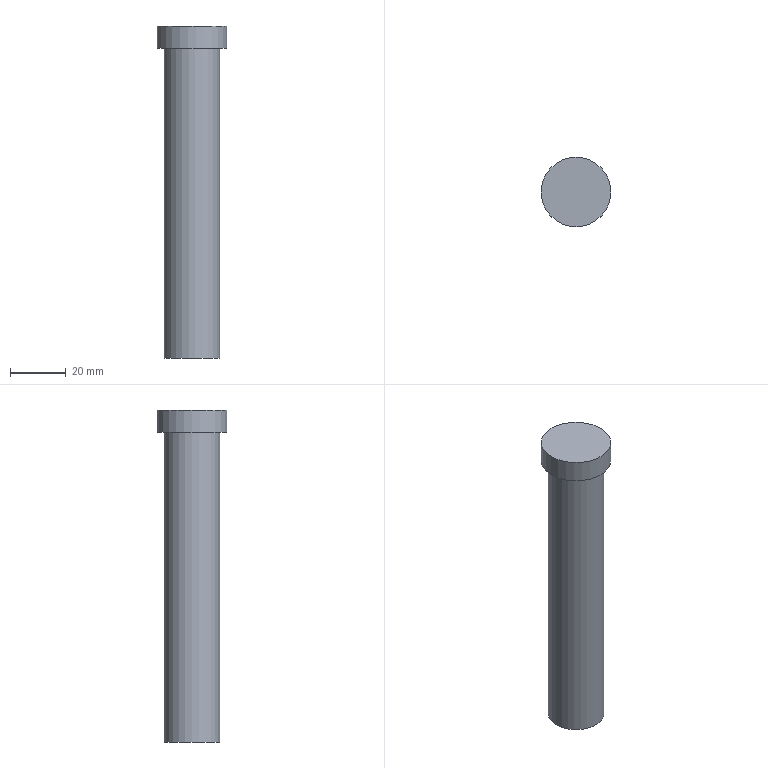Part | STEP file | solid 34 | 1 solid | 8 faces | box 25 x 25 x 119 mm | volume 38365 mm3 | plane 4 | cylinder 3 | cone 1 | commonest cylinder face diameters 6 x1 20 x1 25 x1